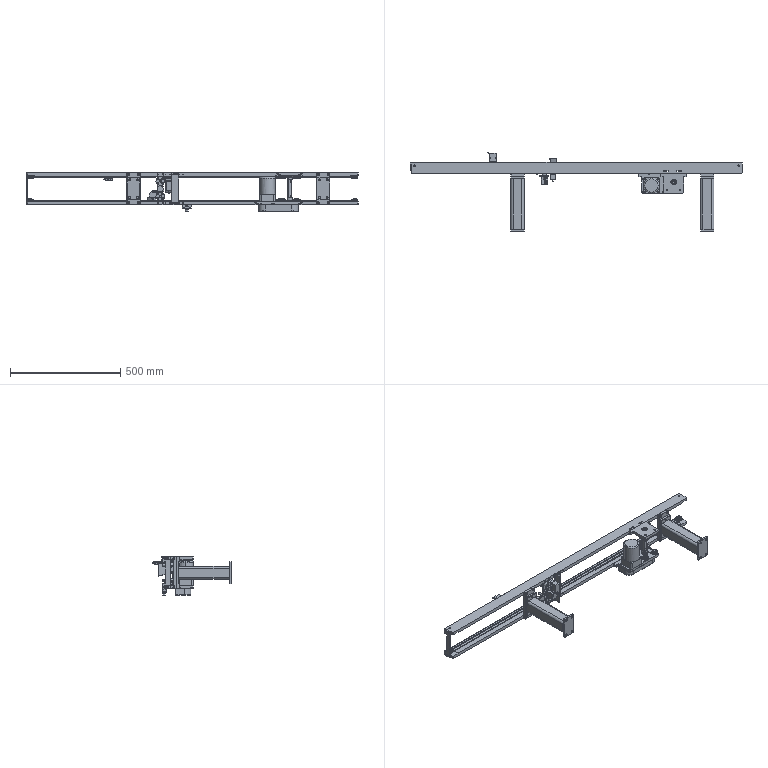Part | SolidWorks | features Belt 2, AEMSimFeature 1, CompositeCurve 1 | 106 solids | 5200 faces | volume 4376702 mm3 | cylinder 1552 | plane 1422 | sphere 1184 | torus 602 | cone 436 | spline 4 | commonest cylinder face diameters 10 x100 0.8 x76 1.2 x76 19 x76 2 x60 27 x56